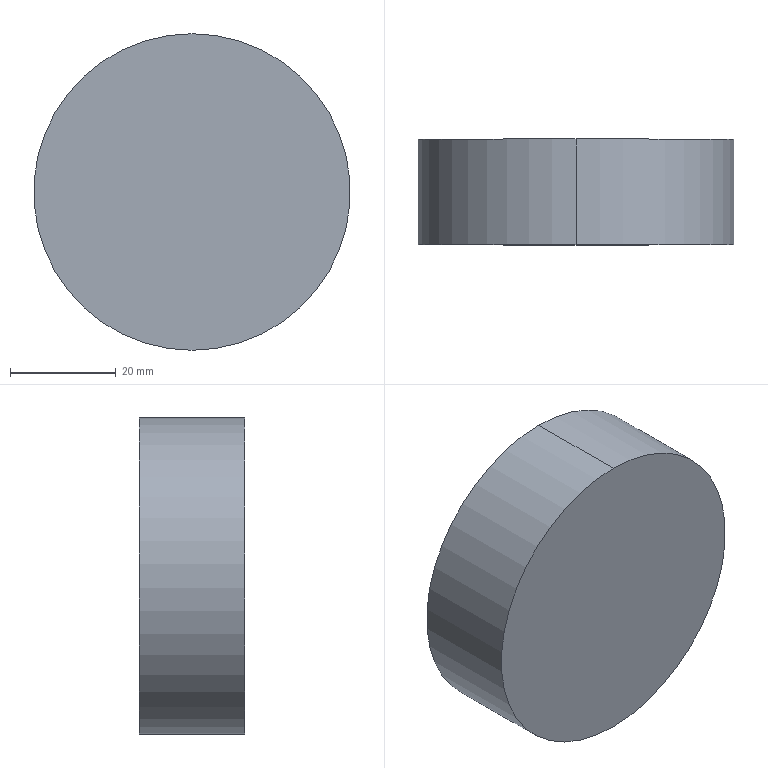Part | 1 solid | 4 faces | box 60 x 20 x 60 mm | volume 56549 mm3 | cylinder 2 | plane 2 | commonest cylinder face diameters 60 x2
STEP:
#1=CARTESIAN_POINT('',(0.,0.,0.));
#2=DIRECTION('',(0.,0.,1.));
#3=DIRECTION('',(1.,0.,0.));
#4=AXIS2_PLACEMENT_3D('',#1,#2,#3);
#5=CARTESIAN_POINT('',(-239.028,-216.5,-330.55));
#6=VERTEX_POINT('',#5);
#7=CARTESIAN_POINT('',(-239.028,-196.5,-330.55));
#8=VERTEX_POINT('',#7);
#9=CARTESIAN_POINT('',(-239.028,-216.5,-330.55));
#10=DIRECTION('',(0.,1.,0.));
#11=VECTOR('',#10,1.);
#12=LINE('',#9,#11);
#13=CARTESIAN_POINT('',(-239.028,-216.5,-300.55));
#14=DIRECTION('',(0.,1.,0.));
#15=DIRECTION('',(1.,0.,0.));
#16=AXIS2_PLACEMENT_3D('',#13,#14,#15);
#17=CYLINDRICAL_SURFACE('',#16,30.);
#18=CARTESIAN_POINT('',(1.571,0.));
#19=DIRECTION('',(0.,1.));
#20=VECTOR('',#19,1.);
#21=LINE('',#18,#20);
#22=(GEOMETRIC_REPRESENTATION_CONTEXT(2)PARAMETRIC_REPRESENTATION_CONTEXT()REPRESENTATION_CONTEXT('',''));
#23=DEFINITIONAL_REPRESENTATION('',(#21),#22);
#24=PCURVE('',#17,#23);
#25=CARTESIAN_POINT('',(-239.028,-216.5,-300.55));
#26=DIRECTION('',(0.,1.,0.));
#27=DIRECTION('',(-1.,0.,0.));
#28=AXIS2_PLACEMENT_3D('',#25,#26,#27);
#29=CYLINDRICAL_SURFACE('',#28,30.);
#30=CARTESIAN_POINT('',(4.712,0.));
#31=DIRECTION('',(0.,1.));
#32=VECTOR('',#31,1.);
#33=LINE('',#30,#32);
#34=(GEOMETRIC_REPRESENTATION_CONTEXT(2)PARAMETRIC_REPRESENTATION_CONTEXT()REPRESENTATION_CONTEXT('',''));
#35=DEFINITIONAL_REPRESENTATION('',(#33),#34);
#36=PCURVE('',#29,#35);
#37=SURFACE_CURVE('',#12,(#24,#36),.PCURVE_S1.);
#38=EDGE_CURVE('',#6,#8,#37,.T.);
#39=ORIENTED_EDGE('',*,*,#38,.F.);
#40=CARTESIAN_POINT('',(-239.028,-216.5,-270.55));
#41=VERTEX_POINT('',#40);
#42=CARTESIAN_POINT('',(-239.028,-216.5,-300.55));
#43=DIRECTION('',(0.,1.,0.));
#44=DIRECTION('',(0.,0.,1.));
#45=AXIS2_PLACEMENT_3D('',#42,#43,#44);
#46=CIRCLE('',#45,30.);
#47=CARTESIAN_POINT('',(-1.571,0.));
#48=DIRECTION('',(1.,0.));
#49=VECTOR('',#48,1.);
#50=LINE('',#47,#49);
#51=(GEOMETRIC_REPRESENTATION_CONTEXT(2)PARAMETRIC_REPRESENTATION_CONTEXT()REPRESENTATION_CONTEXT('',''));
#52=DEFINITIONAL_REPRESENTATION('',(#50),#51);
#53=PCURVE('',#17,#52);
#54=CARTESIAN_POINT('',(-239.028,-216.5,-300.55));
#55=DIRECTION('',(0.,1.,0.));
#56=DIRECTION('',(0.,0.,1.));
#57=AXIS2_PLACEMENT_3D('',#54,#55,#56);
#58=PLANE('',#57);
#59=CARTESIAN_POINT('',(0.,0.));
#60=DIRECTION('',(1.,0.));
#61=AXIS2_PLACEMENT_2D('',#59,#60);
#62=CIRCLE('',#61,30.);
#63=(GEOMETRIC_REPRESENTATION_CONTEXT(2)PARAMETRIC_REPRESENTATION_CONTEXT()REPRESENTATION_CONTEXT('',''));
#64=DEFINITIONAL_REPRESENTATION('',(#62),#63);
#65=PCURVE('',#58,#64);
#66=SURFACE_CURVE('',#46,(#53,#65),.PCURVE_S1.);
#67=EDGE_CURVE('',#6,#41,#66,.T.);
#68=ORIENTED_EDGE('',*,*,#67,.T.);
#69=CARTESIAN_POINT('',(-239.028,-196.5,-270.55));
#70=VERTEX_POINT('',#69);
#71=CARTESIAN_POINT('',(-239.028,-216.5,-270.55));
#72=DIRECTION('',(0.,1.,0.));
#73=VECTOR('',#72,1.);
#74=LINE('',#71,#73);
#75=CARTESIAN_POINT('',(4.712,0.));
#76=DIRECTION('',(0.,1.));
#77=VECTOR('',#76,1.);
#78=LINE('',#75,#77);
#79=(GEOMETRIC_REPRESENTATION_CONTEXT(2)PARAMETRIC_REPRESENTATION_CONTEXT()REPRESENTATION_CONTEXT('',''));
#80=DEFINITIONAL_REPRESENTATION('',(#78),#79);
#81=PCURVE('',#17,#80);
#82=CARTESIAN_POINT('',(1.571,0.));
#83=DIRECTION('',(0.,1.));
#84=VECTOR('',#83,1.);
#85=LINE('',#82,#84);
#86=(GEOMETRIC_REPRESENTATION_CONTEXT(2)PARAMETRIC_REPRESENTATION_CONTEXT()REPRESENTATION_CONTEXT('',''));
#87=DEFINITIONAL_REPRESENTATION('',(#85),#86);
#88=PCURVE('',#29,#87);
#89=SURFACE_CURVE('',#74,(#81,#88),.PCURVE_S1.);
#90=EDGE_CURVE('',#41,#70,#89,.T.);
#91=ORIENTED_EDGE('',*,*,#90,.T.);
#92=CARTESIAN_POINT('',(-239.028,-196.5,-300.55));
#93=DIRECTION('',(0.,1.,0.));
#94=DIRECTION('',(0.,0.,1.));
#95=AXIS2_PLACEMENT_3D('',#92,#93,#94);
#96=CIRCLE('',#95,30.);
#97=CARTESIAN_POINT('',(-1.571,20.));
#98=DIRECTION('',(1.,0.));
#99=VECTOR('',#98,1.);
#100=LINE('',#97,#99);
#101=(GEOMETRIC_REPRESENTATION_CONTEXT(2)PARAMETRIC_REPRESENTATION_CONTEXT()REPRESENTATION_CONTEXT('',''));
#102=DEFINITIONAL_REPRESENTATION('',(#100),#101);
#103=PCURVE('',#17,#102);
#104=CARTESIAN_POINT('',(-239.028,-196.5,-300.55));
#105=DIRECTION('',(0.,1.,0.));
#106=DIRECTION('',(0.,0.,1.));
#107=AXIS2_PLACEMENT_3D('',#104,#105,#106);
#108=PLANE('',#107);
#109=CARTESIAN_POINT('',(0.,0.));
#110=DIRECTION('',(1.,0.));
#111=AXIS2_PLACEMENT_2D('',#109,#110);
#112=CIRCLE('',#111,30.);
#113=(GEOMETRIC_REPRESENTATION_CONTEXT(2)PARAMETRIC_REPRESENTATION_CONTEXT()REPRESENTATION_CONTEXT('',''));
#114=DEFINITIONAL_REPRESENTATION('',(#112),#113);
#115=PCURVE('',#108,#114);
#116=SURFACE_CURVE('',#96,(#103,#115),.PCURVE_S1.);
#117=EDGE_CURVE('',#8,#70,#116,.T.);
#118=ORIENTED_EDGE('',*,*,#117,.F.);
#119=EDGE_LOOP('',(#39,#68,#91,#118));
#120=FACE_BOUND('',#119,.T.);
#121=ADVANCED_FACE('',(#120),#17,.T.);
#122=CARTESIAN_POINT('',(-239.028,-196.5,-300.55));
#123=DIRECTION('',(0.,1.,0.));
#124=DIRECTION('',(0.,0.,1.));
#125=AXIS2_PLACEMENT_3D('',#122,#123,#124);
#126=CIRCLE('',#125,30.);
#127=CARTESIAN_POINT('',(0.,0.));
#128=DIRECTION('',(1.,0.));
#129=AXIS2_PLACEMENT_2D('',#127,#128);
#130=CIRCLE('',#129,30.);
#131=(GEOMETRIC_REPRESENTATION_CONTEXT(2)PARAMETRIC_REPRESENTATION_CONTEXT()REPRESENTATION_CONTEXT('',''));
#132=DEFINITIONAL_REPRESENTATION('',(#130),#131);
#133=PCURVE('',#108,#132);
#134=CARTESIAN_POINT('',(1.571,20.));
#135=DIRECTION('',(1.,0.));
#136=VECTOR('',#135,1.);
#137=LINE('',#134,#136);
#138=(GEOMETRIC_REPRESENTATION_CONTEXT(2)PARAMETRIC_REPRESENTATION_CONTEXT()REPRESENTATION_CONTEXT('',''));
#139=DEFINITIONAL_REPRESENTATION('',(#137),#138);
#140=PCURVE('',#29,#139);
#141=SURFACE_CURVE('',#126,(#133,#140),.PCURVE_S1.);
#142=EDGE_CURVE('',#70,#8,#141,.T.);
#143=ORIENTED_EDGE('',*,*,#142,.T.);
#144=ORIENTED_EDGE('',*,*,#117,.T.);
#145=EDGE_LOOP('',(#143,#144));
#146=FACE_BOUND('',#145,.T.);
#147=ADVANCED_FACE('',(#146),#108,.T.);
#148=ORIENTED_EDGE('',*,*,#67,.F.);
#149=CARTESIAN_POINT('',(-239.028,-216.5,-300.55));
#150=DIRECTION('',(0.,1.,0.));
#151=DIRECTION('',(0.,0.,1.));
#152=AXIS2_PLACEMENT_3D('',#149,#150,#151);
#153=CIRCLE('',#152,30.);
#154=CARTESIAN_POINT('',(0.,0.));
#155=DIRECTION('',(1.,0.));
#156=AXIS2_PLACEMENT_2D('',#154,#155);
#157=CIRCLE('',#156,30.);
#158=(GEOMETRIC_REPRESENTATION_CONTEXT(2)PARAMETRIC_REPRESENTATION_CONTEXT()REPRESENTATION_CONTEXT('',''));
#159=DEFINITIONAL_REPRESENTATION('',(#157),#158);
#160=PCURVE('',#58,#159);
#161=CARTESIAN_POINT('',(1.571,0.));
#162=DIRECTION('',(1.,0.));
#163=VECTOR('',#162,1.);
#164=LINE('',#161,#163);
#165=(GEOMETRIC_REPRESENTATION_CONTEXT(2)PARAMETRIC_REPRESENTATION_CONTEXT()REPRESENTATION_CONTEXT('',''));
#166=DEFINITIONAL_REPRESENTATION('',(#164),#165);
#167=PCURVE('',#29,#166);
#168=SURFACE_CURVE('',#153,(#160,#167),.PCURVE_S1.);
#169=EDGE_CURVE('',#41,#6,#168,.T.);
#170=ORIENTED_EDGE('',*,*,#169,.F.);
#171=EDGE_LOOP('',(#148,#170));
#172=FACE_BOUND('',#171,.T.);
#173=ADVANCED_FACE('',(#172),#58,.F.);
#174=ORIENTED_EDGE('',*,*,#38,.T.);
#175=ORIENTED_EDGE('',*,*,#142,.F.);
#176=ORIENTED_EDGE('',*,*,#90,.F.);
#177=ORIENTED_EDGE('',*,*,#169,.T.);
#178=EDGE_LOOP('',(#174,#175,#176,#177));
#179=FACE_BOUND('',#178,.T.);
#180=ADVANCED_FACE('',(#179),#29,.T.);
#181=CLOSED_SHELL('',(#121,#147,#173,#180));
#182=MANIFOLD_SOLID_BREP('',#181);
#183=(LENGTH_UNIT()NAMED_UNIT(*)SI_UNIT(.MILLI.,.METRE.));
#184=UNCERTAINTY_MEASURE_WITH_UNIT(LENGTH_MEASURE(0.0000001),#183,'','');
#185=(NAMED_UNIT(*)PLANE_ANGLE_UNIT()SI_UNIT($,.RADIAN.));
#186=(NAMED_UNIT(*)SI_UNIT($,.STERADIAN.)SOLID_ANGLE_UNIT());
#187=(GEOMETRIC_REPRESENTATION_CONTEXT(3)GLOBAL_UNCERTAINTY_ASSIGNED_CONTEXT((#184))GLOBAL_UNIT_ASSIGNED_CONTEXT((#183,#185,#186))REPRESENTATION_CONTEXT('',''));
#188=ADVANCED_BREP_SHAPE_REPRESENTATION('',(#4,#182),#187);